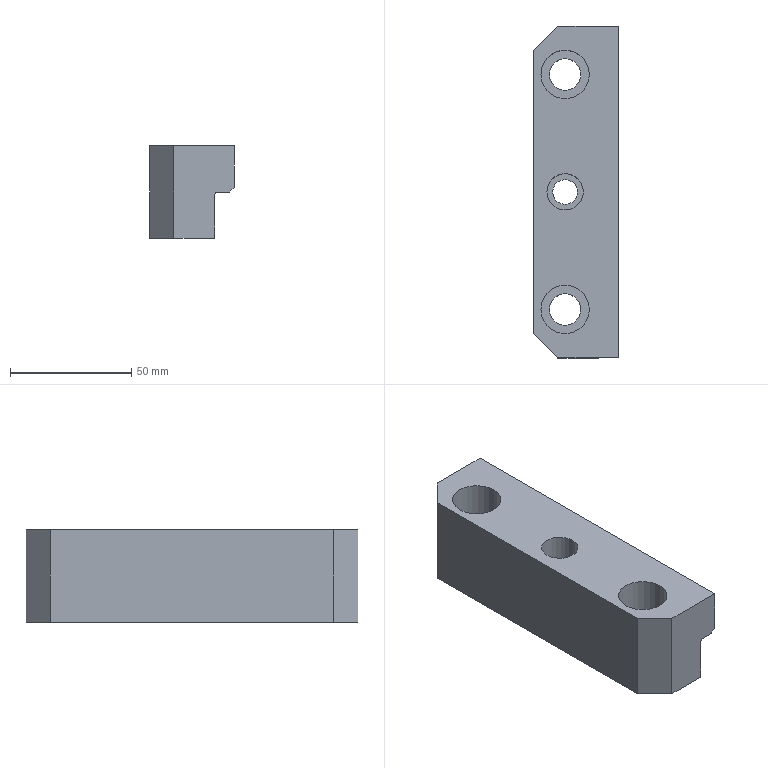Part | STEP file | 1_id626_x_t | 1 solid | 21 faces | box 35 x 137 x 38.1 mm | volume 136243 mm3 | plane 14 | cylinder 7 | commonest cylinder face diameters 13 x2 20 x2 3 x1 10.25 x1 15 x1